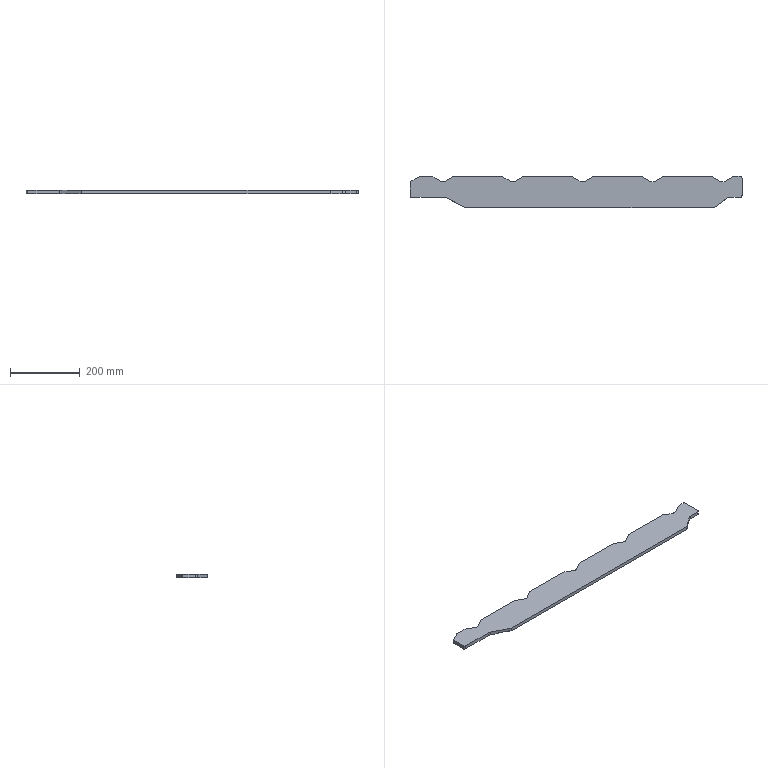Part | STEP file | 001-008-Traverse module transfer fixture | 1 solid | 42 faces | box 950 x 90 x 10 mm | volume 745703 mm3 | plane 30 | cylinder 12 | commonest cylinder face diameters 30 x7 10 x5